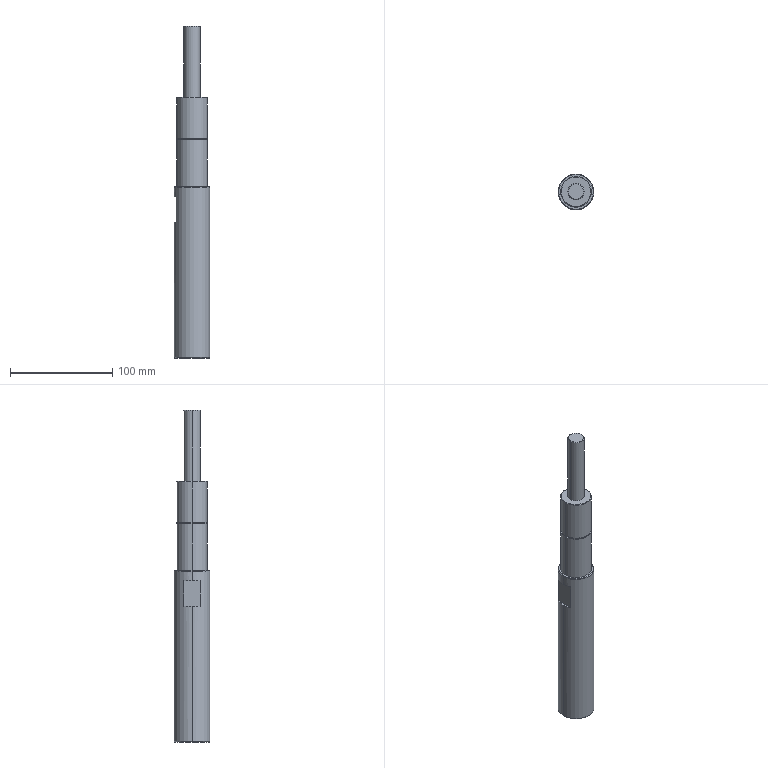Part | STEP file | 2086 Fixed shaft | 1 solid | 27 faces | box 35 x 35 x 325.3 mm | volume 236741 mm3 | cylinder 10 | plane 9 | cone 8 | commonest cylinder face diameters 30 x4 16 x2 28.6 x2 35 x2